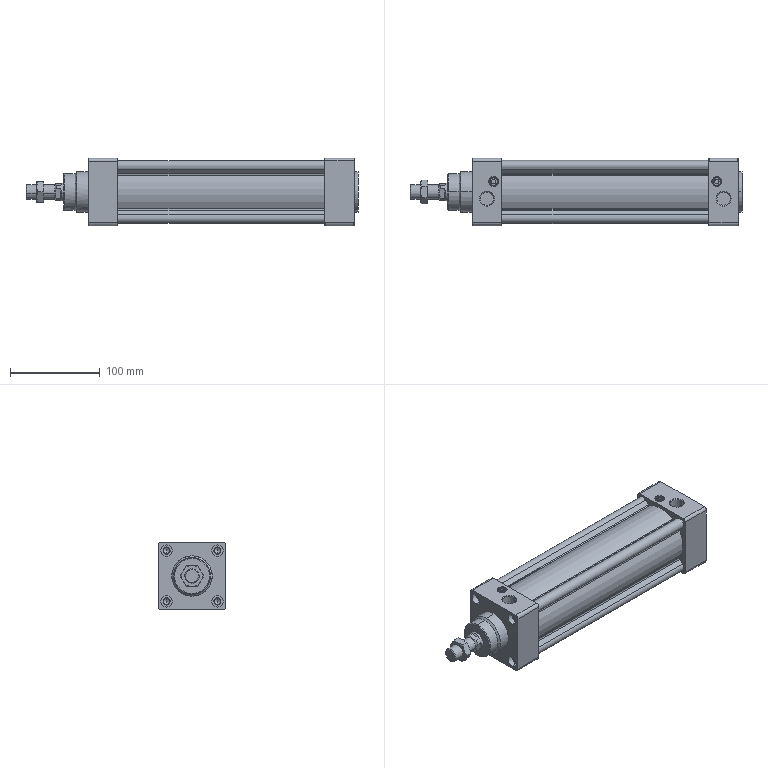Part | SolidWorks | 3 solids | 256 faces | box 369 x 75 x 75 mm | volume 826991 mm3 | cylinder 107 | plane 77 | cone 70 | spline 2 | commonest cylinder face diameters 6.647 x16 12.7 x16 4 x10 6.8 x8 7 x6 12 x6